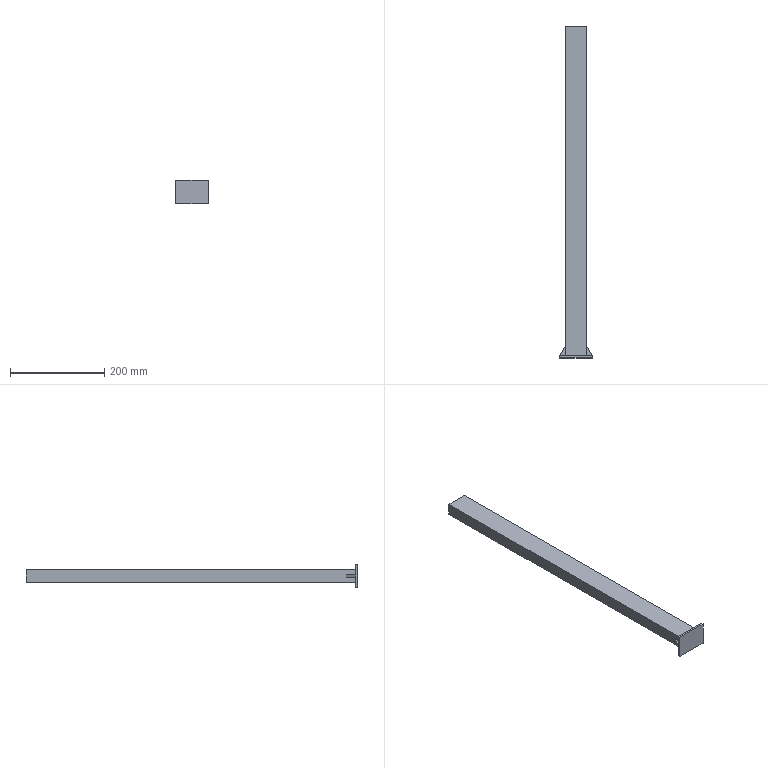Part | SolidWorks | features ICE 3, Extrusion 1 | 1 solid | 23 faces | box 70 x 705 x 50 mm | volume 217416 mm3 | plane 23
STEP:
#1=CARTESIAN_POINT('',(-415.,5.,25.));
#2=VERTEX_POINT('',#1);
#3=CARTESIAN_POINT('',(-415.,5.,2.5));
#4=VERTEX_POINT('',#3);
#5=CARTESIAN_POINT('',(-415.,5.,-25.));
#6=DIRECTION('',(0.,0.,-1.));
#7=VECTOR('',#6,1000.);
#8=LINE('',#5,#7);
#9=EDGE_CURVE('',#2,#4,#8,.T.);
#10=ORIENTED_EDGE('',*,*,#9,.T.);
#11=CARTESIAN_POINT('',(-427.,5.,2.5));
#12=VERTEX_POINT('',#11);
#13=CARTESIAN_POINT('',(-427.,5.,2.5));
#14=DIRECTION('',(1.,0.,0.));
#15=VECTOR('',#14,1000.);
#16=LINE('',#13,#15);
#17=EDGE_CURVE('',#12,#4,#16,.T.);
#18=ORIENTED_EDGE('',*,*,#17,.F.);
#19=CARTESIAN_POINT('',(-427.,5.,13.));
#20=VERTEX_POINT('',#19);
#21=CARTESIAN_POINT('',(-427.,5.,13.));
#22=DIRECTION('',(0.,0.,-1.));
#23=VECTOR('',#22,1000.);
#24=LINE('',#21,#23);
#25=EDGE_CURVE('',#20,#12,#24,.T.);
#26=ORIENTED_EDGE('',*,*,#25,.F.);
#27=CARTESIAN_POINT('',(-473.,5.,13.));
#28=VERTEX_POINT('',#27);
#29=CARTESIAN_POINT('',(-473.,5.,13.));
#30=DIRECTION('',(1.,0.,0.));
#31=VECTOR('',#30,1000.);
#32=LINE('',#29,#31);
#33=EDGE_CURVE('',#28,#20,#32,.T.);
#34=ORIENTED_EDGE('',*,*,#33,.F.);
#35=CARTESIAN_POINT('',(-473.,5.,2.5));
#36=VERTEX_POINT('',#35);
#37=CARTESIAN_POINT('',(-473.,5.,-13.));
#38=DIRECTION('',(0.,0.,1.));
#39=VECTOR('',#38,1000.);
#40=LINE('',#37,#39);
#41=EDGE_CURVE('',#36,#28,#40,.T.);
#42=ORIENTED_EDGE('',*,*,#41,.F.);
#43=CARTESIAN_POINT('',(-485.,5.,2.5));
#44=VERTEX_POINT('',#43);
#45=CARTESIAN_POINT('',(-473.,5.,2.5));
#46=DIRECTION('',(1.,0.,0.));
#47=VECTOR('',#46,1000.);
#48=LINE('',#45,#47);
#49=EDGE_CURVE('',#44,#36,#48,.T.);
#50=ORIENTED_EDGE('',*,*,#49,.F.);
#51=CARTESIAN_POINT('',(-485.,5.,25.));
#52=VERTEX_POINT('',#51);
#53=CARTESIAN_POINT('',(-485.,5.,-25.));
#54=DIRECTION('',(0.,0.,1.));
#55=VECTOR('',#54,1000.);
#56=LINE('',#53,#55);
#57=EDGE_CURVE('',#44,#52,#56,.T.);
#58=ORIENTED_EDGE('',*,*,#57,.T.);
#59=CARTESIAN_POINT('',(-485.,5.,25.));
#60=DIRECTION('',(1.,0.,0.));
#61=VECTOR('',#60,1000.);
#62=LINE('',#59,#61);
#63=EDGE_CURVE('',#52,#2,#62,.T.);
#64=ORIENTED_EDGE('',*,*,#63,.T.);
#65=EDGE_LOOP('',(#10,#18,#26,#34,#42,#50,#58,#64));
#66=FACE_OUTER_BOUND('',#65,.T.);
#67=CARTESIAN_POINT('',(0.,5.,0.));
#68=DIRECTION('',(0.,1.,0.));
#69=DIRECTION('',(0.,0.,1.));
#70=AXIS2_PLACEMENT_3D('',#67,#68,#69);
#71=PLANE('',#70);
#72=ADVANCED_FACE('',(#66),#71,.T.);
#73=CARTESIAN_POINT('',(-427.,25.,2.5));
#74=VERTEX_POINT('',#73);
#75=CARTESIAN_POINT('',(-427.,25.,2.5));
#76=DIRECTION('',(0.,-1.,0.));
#77=VECTOR('',#76,1000.);
#78=LINE('',#75,#77);
#79=EDGE_CURVE('',#74,#12,#78,.T.);
#80=ORIENTED_EDGE('',*,*,#79,.F.);
#81=CARTESIAN_POINT('',(-427.,25.,-2.5));
#82=VERTEX_POINT('',#81);
#83=CARTESIAN_POINT('',(-427.,25.,2.5));
#84=DIRECTION('',(0.,0.,-1.));
#85=VECTOR('',#84,1000.);
#86=LINE('',#83,#85);
#87=EDGE_CURVE('',#74,#82,#86,.T.);
#88=ORIENTED_EDGE('',*,*,#87,.T.);
#89=CARTESIAN_POINT('',(-427.,5.,-2.5));
#90=VERTEX_POINT('',#89);
#91=CARTESIAN_POINT('',(-427.,25.,-2.5));
#92=DIRECTION('',(0.,-1.,0.));
#93=VECTOR('',#92,1000.);
#94=LINE('',#91,#93);
#95=EDGE_CURVE('',#82,#90,#94,.T.);
#96=ORIENTED_EDGE('',*,*,#95,.T.);
#97=CARTESIAN_POINT('',(-427.,5.,-13.));
#98=VERTEX_POINT('',#97);
#99=CARTESIAN_POINT('',(-427.,5.,13.));
#100=DIRECTION('',(0.,0.,-1.));
#101=VECTOR('',#100,1000.);
#102=LINE('',#99,#101);
#103=EDGE_CURVE('',#90,#98,#102,.T.);
#104=ORIENTED_EDGE('',*,*,#103,.T.);
#105=CARTESIAN_POINT('',(-427.,705.,-13.));
#106=VERTEX_POINT('',#105);
#107=CARTESIAN_POINT('',(-427.,705.,-13.));
#108=DIRECTION('',(0.,-1.,0.));
#109=VECTOR('',#108,1000.);
#110=LINE('',#107,#109);
#111=EDGE_CURVE('',#106,#98,#110,.T.);
#112=ORIENTED_EDGE('',*,*,#111,.F.);
#113=CARTESIAN_POINT('',(-427.,705.,13.));
#114=VERTEX_POINT('',#113);
#115=CARTESIAN_POINT('',(-427.,705.,13.));
#116=DIRECTION('',(0.,0.,-1.));
#117=VECTOR('',#116,1000.);
#118=LINE('',#115,#117);
#119=EDGE_CURVE('',#114,#106,#118,.T.);
#120=ORIENTED_EDGE('',*,*,#119,.F.);
#121=CARTESIAN_POINT('',(-427.,705.,13.));
#122=DIRECTION('',(0.,-1.,0.));
#123=VECTOR('',#122,1000.);
#124=LINE('',#121,#123);
#125=EDGE_CURVE('',#114,#20,#124,.T.);
#126=ORIENTED_EDGE('',*,*,#125,.T.);
#127=ORIENTED_EDGE('',*,*,#25,.T.);
#128=EDGE_LOOP('',(#80,#88,#96,#104,#112,#120,#126,#127));
#129=FACE_OUTER_BOUND('',#128,.T.);
#130=CARTESIAN_POINT('',(-427.,705.,13.));
#131=DIRECTION('',(-1.,0.,0.));
#132=DIRECTION('',(0.,0.,1.));
#133=AXIS2_PLACEMENT_3D('',#130,#131,#132);
#134=PLANE('',#133);
#135=ADVANCED_FACE('',(#129),#134,.F.);
#136=CARTESIAN_POINT('',(-415.,5.,-2.5));
#137=VERTEX_POINT('',#136);
#138=CARTESIAN_POINT('',(-427.,5.,-2.5));
#139=DIRECTION('',(1.,0.,0.));
#140=VECTOR('',#139,1000.);
#141=LINE('',#138,#140);
#142=EDGE_CURVE('',#90,#137,#141,.T.);
#143=ORIENTED_EDGE('',*,*,#142,.T.);
#144=CARTESIAN_POINT('',(-415.,5.,-25.));
#145=VERTEX_POINT('',#144);
#146=CARTESIAN_POINT('',(-415.,5.,-25.));
#147=DIRECTION('',(0.,0.,-1.));
#148=VECTOR('',#147,1000.);
#149=LINE('',#146,#148);
#150=EDGE_CURVE('',#137,#145,#149,.T.);
#151=ORIENTED_EDGE('',*,*,#150,.T.);
#152=CARTESIAN_POINT('',(-485.,5.,-25.));
#153=VERTEX_POINT('',#152);
#154=CARTESIAN_POINT('',(-485.,5.,-25.));
#155=DIRECTION('',(-1.,0.,0.));
#156=VECTOR('',#155,1000.);
#157=LINE('',#154,#156);
#158=EDGE_CURVE('',#145,#153,#157,.T.);
#159=ORIENTED_EDGE('',*,*,#158,.T.);
#160=CARTESIAN_POINT('',(-485.,5.,-2.5));
#161=VERTEX_POINT('',#160);
#162=CARTESIAN_POINT('',(-485.,5.,-25.));
#163=DIRECTION('',(0.,0.,1.));
#164=VECTOR('',#163,1000.);
#165=LINE('',#162,#164);
#166=EDGE_CURVE('',#153,#161,#165,.T.);
#167=ORIENTED_EDGE('',*,*,#166,.T.);
#168=CARTESIAN_POINT('',(-473.,5.,-2.5));
#169=VERTEX_POINT('',#168);
#170=CARTESIAN_POINT('',(-473.,5.,-2.5));
#171=DIRECTION('',(1.,0.,0.));
#172=VECTOR('',#171,1000.);
#173=LINE('',#170,#172);
#174=EDGE_CURVE('',#161,#169,#173,.T.);
#175=ORIENTED_EDGE('',*,*,#174,.T.);
#176=CARTESIAN_POINT('',(-473.,5.,-13.));
#177=VERTEX_POINT('',#176);
#178=CARTESIAN_POINT('',(-473.,5.,-13.));
#179=DIRECTION('',(0.,0.,1.));
#180=VECTOR('',#179,1000.);
#181=LINE('',#178,#180);
#182=EDGE_CURVE('',#177,#169,#181,.T.);
#183=ORIENTED_EDGE('',*,*,#182,.F.);
#184=CARTESIAN_POINT('',(-427.,5.,-13.));
#185=DIRECTION('',(-1.,0.,0.));
#186=VECTOR('',#185,1000.);
#187=LINE('',#184,#186);
#188=EDGE_CURVE('',#98,#177,#187,.T.);
#189=ORIENTED_EDGE('',*,*,#188,.F.);
#190=ORIENTED_EDGE('',*,*,#103,.F.);
#191=EDGE_LOOP('',(#143,#151,#159,#167,#175,#183,#189,#190));
#192=FACE_OUTER_BOUND('',#191,.T.);
#193=CARTESIAN_POINT('',(0.,5.,0.));
#194=DIRECTION('',(0.,1.,0.));
#195=DIRECTION('',(0.,0.,1.));
#196=AXIS2_PLACEMENT_3D('',#193,#194,#195);
#197=PLANE('',#196);
#198=ADVANCED_FACE('',(#192),#197,.T.);
#199=CARTESIAN_POINT('',(-473.,25.,2.5));
#200=VERTEX_POINT('',#199);
#201=CARTESIAN_POINT('',(-473.,25.,2.5));
#202=DIRECTION('',(0.,1.,0.));
#203=VECTOR('',#202,1000.);
#204=LINE('',#201,#203);
#205=EDGE_CURVE('',#36,#200,#204,.T.);
#206=ORIENTED_EDGE('',*,*,#205,.F.);
#207=ORIENTED_EDGE('',*,*,#41,.T.);
#208=CARTESIAN_POINT('',(-473.,705.,13.));
#209=VERTEX_POINT('',#208);
#210=CARTESIAN_POINT('',(-473.,705.,13.));
#211=DIRECTION('',(0.,-1.,0.));
#212=VECTOR('',#211,1000.);
#213=LINE('',#210,#212);
#214=EDGE_CURVE('',#209,#28,#213,.T.);
#215=ORIENTED_EDGE('',*,*,#214,.F.);
#216=CARTESIAN_POINT('',(-473.,705.,-13.));
#217=VERTEX_POINT('',#216);
#218=CARTESIAN_POINT('',(-473.,705.,-13.));
#219=DIRECTION('',(0.,0.,1.));
#220=VECTOR('',#219,1000.);
#221=LINE('',#218,#220);
#222=EDGE_CURVE('',#217,#209,#221,.T.);
#223=ORIENTED_EDGE('',*,*,#222,.F.);
#224=CARTESIAN_POINT('',(-473.,705.,-13.));
#225=DIRECTION('',(0.,-1.,0.));
#226=VECTOR('',#225,1000.);
#227=LINE('',#224,#226);
#228=EDGE_CURVE('',#217,#177,#227,.T.);
#229=ORIENTED_EDGE('',*,*,#228,.T.);
#230=ORIENTED_EDGE('',*,*,#182,.T.);
#231=CARTESIAN_POINT('',(-473.,25.,-2.5));
#232=VERTEX_POINT('',#231);
#233=CARTESIAN_POINT('',(-473.,25.,-2.5));
#234=DIRECTION('',(0.,1.,0.));
#235=VECTOR('',#234,1000.);
#236=LINE('',#233,#235);
#237=EDGE_CURVE('',#169,#232,#236,.T.);
#238=ORIENTED_EDGE('',*,*,#237,.T.);
#239=CARTESIAN_POINT('',(-473.,25.,2.5));
#240=DIRECTION('',(0.,0.,-1.));
#241=VECTOR('',#240,1000.);
#242=LINE('',#239,#241);
#243=EDGE_CURVE('',#200,#232,#242,.T.);
#244=ORIENTED_EDGE('',*,*,#243,.F.);
#245=EDGE_LOOP('',(#206,#207,#215,#223,#229,#230,#238,#244));
#246=FACE_OUTER_BOUND('',#245,.T.);
#247=CARTESIAN_POINT('',(-473.,705.,-13.));
#248=DIRECTION('',(1.,0.,0.));
#249=DIRECTION('',(0.,0.,-1.));
#250=AXIS2_PLACEMENT_3D('',#247,#248,#249);
#251=PLANE('',#250);
#252=ADVANCED_FACE('',(#246),#251,.F.);
#253=CARTESIAN_POINT('',(-415.,0.,25.));
#254=VERTEX_POINT('',#253);
#255=CARTESIAN_POINT('',(-415.,0.,-25.));
#256=VERTEX_POINT('',#255);
#257=CARTESIAN_POINT('',(-415.,0.,-25.));
#258=DIRECTION('',(0.,0.,-1.));
#259=VECTOR('',#258,1000.);
#260=LINE('',#257,#259);
#261=EDGE_CURVE('',#254,#256,#260,.T.);
#262=ORIENTED_EDGE('',*,*,#261,.T.);
#263=CARTESIAN_POINT('',(-415.,5.,-25.));
#264=DIRECTION('',(0.,-1.,0.));
#265=VECTOR('',#264,1000.);
#266=LINE('',#263,#265);
#267=EDGE_CURVE('',#145,#256,#266,.T.);
#268=ORIENTED_EDGE('',*,*,#267,.F.);
#269=ORIENTED_EDGE('',*,*,#150,.F.);
#270=CARTESIAN_POINT('',(-415.,5.,2.5));
#271=DIRECTION('',(0.,0.,-1.));
#272=VECTOR('',#271,1000.);
#273=LINE('',#270,#272);
#274=EDGE_CURVE('',#4,#137,#273,.T.);
#275=ORIENTED_EDGE('',*,*,#274,.F.);
#276=ORIENTED_EDGE('',*,*,#9,.F.);
#277=CARTESIAN_POINT('',(-415.,5.,25.));
#278=DIRECTION('',(0.,-1.,0.));
#279=VECTOR('',#278,1000.);
#280=LINE('',#277,#279);
#281=EDGE_CURVE('',#2,#254,#280,.T.);
#282=ORIENTED_EDGE('',*,*,#281,.T.);
#283=EDGE_LOOP('',(#262,#268,#269,#275,#276,#282));
#284=FACE_OUTER_BOUND('',#283,.T.);
#285=CARTESIAN_POINT('',(-415.,5.,-25.));
#286=DIRECTION('',(-1.,0.,0.));
#287=DIRECTION('',(0.,0.,1.));
#288=AXIS2_PLACEMENT_3D('',#285,#286,#287);
#289=PLANE('',#288);
#290=ADVANCED_FACE('',(#284),#289,.F.);
#291=CARTESIAN_POINT('',(-485.,0.,-25.));
#292=VERTEX_POINT('',#291);
#293=CARTESIAN_POINT('',(-485.,0.,-25.));
#294=DIRECTION('',(-1.,0.,0.));
#295=VECTOR('',#294,1000.);
#296=LINE('',#293,#295);
#297=EDGE_CURVE('',#256,#292,#296,.T.);
#298=ORIENTED_EDGE('',*,*,#297,.T.);
#299=CARTESIAN_POINT('',(-485.,5.,-25.));
#300=DIRECTION('',(0.,-1.,0.));
#301=VECTOR('',#300,1000.);
#302=LINE('',#299,#301);
#303=EDGE_CURVE('',#153,#292,#302,.T.);
#304=ORIENTED_EDGE('',*,*,#303,.F.);
#305=ORIENTED_EDGE('',*,*,#158,.F.);
#306=ORIENTED_EDGE('',*,*,#267,.T.);
#307=EDGE_LOOP('',(#298,#304,#305,#306));
#308=FACE_OUTER_BOUND('',#307,.T.);
#309=CARTESIAN_POINT('',(-485.,5.,-25.));
#310=DIRECTION('',(0.,0.,1.));
#311=DIRECTION('',(1.,0.,0.));
#312=AXIS2_PLACEMENT_3D('',#309,#310,#311);
#313=PLANE('',#312);
#314=ADVANCED_FACE('',(#308),#313,.F.);
#315=CARTESIAN_POINT('',(-485.,0.,25.));
#316=VERTEX_POINT('',#315);
#317=CARTESIAN_POINT('',(-485.,0.,-25.));
#318=DIRECTION('',(0.,0.,1.));
#319=VECTOR('',#318,1000.);
#320=LINE('',#317,#319);
#321=EDGE_CURVE('',#292,#316,#320,.T.);
#322=ORIENTED_EDGE('',*,*,#321,.T.);
#323=CARTESIAN_POINT('',(-485.,5.,25.));
#324=DIRECTION('',(0.,-1.,0.));
#325=VECTOR('',#324,1000.);
#326=LINE('',#323,#325);
#327=EDGE_CURVE('',#52,#316,#326,.T.);
#328=ORIENTED_EDGE('',*,*,#327,.F.);
#329=ORIENTED_EDGE('',*,*,#57,.F.);
#330=CARTESIAN_POINT('',(-485.,5.,2.5));
#331=DIRECTION('',(0.,0.,-1.));
#332=VECTOR('',#331,1000.);
#333=LINE('',#330,#332);
#334=EDGE_CURVE('',#44,#161,#333,.T.);
#335=ORIENTED_EDGE('',*,*,#334,.T.);
#336=ORIENTED_EDGE('',*,*,#166,.F.);
#337=ORIENTED_EDGE('',*,*,#303,.T.);
#338=EDGE_LOOP('',(#322,#328,#329,#335,#336,#337));
#339=FACE_OUTER_BOUND('',#338,.T.);
#340=CARTESIAN_POINT('',(-485.,5.,-25.));
#341=DIRECTION('',(1.,0.,0.));
#342=DIRECTION('',(0.,0.,-1.));
#343=AXIS2_PLACEMENT_3D('',#340,#341,#342);
#344=PLANE('',#343);
#345=ADVANCED_FACE('',(#339),#344,.F.);
#346=CARTESIAN_POINT('',(-485.,0.,25.));
#347=DIRECTION('',(1.,0.,0.));
#348=VECTOR('',#347,1000.);
#349=LINE('',#346,#348);
#350=EDGE_CURVE('',#316,#254,#349,.T.);
#351=ORIENTED_EDGE('',*,*,#350,.T.);
#352=ORIENTED_EDGE('',*,*,#281,.F.);
#353=ORIENTED_EDGE('',*,*,#63,.F.);
#354=ORIENTED_EDGE('',*,*,#327,.T.);
#355=EDGE_LOOP('',(#351,#352,#353,#354));
#356=FACE_OUTER_BOUND('',#355,.T.);
#357=CARTESIAN_POINT('',(-485.,5.,25.));
#358=DIRECTION('',(0.,0.,-1.));
#359=DIRECTION('',(-1.,0.,0.));
#360=AXIS2_PLACEMENT_3D('',#357,#358,#359);
#361=PLANE('',#360);
#362=ADVANCED_FACE('',(#356),#361,.F.);
#363=ORIENTED_EDGE('',*,*,#261,.F.);
#364=ORIENTED_EDGE('',*,*,#350,.F.);
#365=ORIENTED_EDGE('',*,*,#321,.F.);
#366=ORIENTED_EDGE('',*,*,#297,.F.);
#367=EDGE_LOOP('',(#363,#364,#365,#366));
#368=FACE_OUTER_BOUND('',#367,.T.);
#369=CARTESIAN_POINT('',(0.,0.,0.));
#370=DIRECTION('',(0.,1.,0.));
#371=DIRECTION('',(0.,0.,1.));
#372=AXIS2_PLACEMENT_3D('',#369,#370,#371);
#373=PLANE('',#372);
#374=ADVANCED_FACE('',(#368),#373,.F.);
#375=ORIENTED_EDGE('',*,*,#33,.T.);
#376=ORIENTED_EDGE('',*,*,#125,.F.);
#377=CARTESIAN_POINT('',(-473.,705.,13.));
#378=DIRECTION('',(1.,0.,0.));
#379=VECTOR('',#378,1000.);
#380=LINE('',#377,#379);
#381=EDGE_CURVE('',#209,#114,#380,.T.);
#382=ORIENTED_EDGE('',*,*,#381,.F.);
#383=ORIENTED_EDGE('',*,*,#214,.T.);
#384=EDGE_LOOP('',(#375,#376,#382,#383));
#385=FACE_OUTER_BOUND('',#384,.T.);
#386=CARTESIAN_POINT('',(-473.,705.,13.));
#387=DIRECTION('',(0.,0.,-1.));
#388=DIRECTION('',(-1.,0.,0.));
#389=AXIS2_PLACEMENT_3D('',#386,#387,#388);
#390=PLANE('',#389);
#391=ADVANCED_FACE('',(#385),#390,.F.);
#392=ORIENTED_EDGE('',*,*,#188,.T.);
#393=ORIENTED_EDGE('',*,*,#228,.F.);
#394=CARTESIAN_POINT('',(-427.,705.,-13.));
#395=DIRECTION('',(-1.,0.,0.));
#396=VECTOR('',#395,1000.);
#397=LINE('',#394,#396);
#398=EDGE_CURVE('',#106,#217,#397,.T.);
#399=ORIENTED_EDGE('',*,*,#398,.F.);
#400=ORIENTED_EDGE('',*,*,#111,.T.);
#401=EDGE_LOOP('',(#392,#393,#399,#400));
#402=FACE_OUTER_BOUND('',#401,.T.);
#403=CARTESIAN_POINT('',(-427.,705.,-13.));
#404=DIRECTION('',(0.,0.,1.));
#405=DIRECTION('',(1.,0.,0.));
#406=AXIS2_PLACEMENT_3D('',#403,#404,#405);
#407=PLANE('',#406);
#408=ADVANCED_FACE('',(#402),#407,.F.);
#409=CARTESIAN_POINT('',(-471.,705.,-11.));
#410=VERTEX_POINT('',#409);
#411=CARTESIAN_POINT('',(-471.,705.,11.));
#412=VERTEX_POINT('',#411);
#413=CARTESIAN_POINT('',(-471.,705.,-11.));
#414=DIRECTION('',(0.,0.,1.));
#415=VECTOR('',#414,1000.);
#416=LINE('',#413,#415);
#417=EDGE_CURVE('',#410,#412,#416,.T.);
#418=ORIENTED_EDGE('',*,*,#417,.F.);
#419=CARTESIAN_POINT('',(-429.,705.,-11.));
#420=VERTEX_POINT('',#419);
#421=CARTESIAN_POINT('',(-429.,705.,-11.));
#422=DIRECTION('',(-1.,0.,0.));
#423=VECTOR('',#422,1000.);
#424=LINE('',#421,#423);
#425=EDGE_CURVE('',#420,#410,#424,.T.);
#426=ORIENTED_EDGE('',*,*,#425,.F.);
#427=CARTESIAN_POINT('',(-429.,705.,11.));
#428=VERTEX_POINT('',#427);
#429=CARTESIAN_POINT('',(-429.,705.,11.));
#430=DIRECTION('',(0.,0.,-1.));
#431=VECTOR('',#430,1000.);
#432=LINE('',#429,#431);
#433=EDGE_CURVE('',#428,#420,#432,.T.);
#434=ORIENTED_EDGE('',*,*,#433,.F.);
#435=CARTESIAN_POINT('',(-471.,705.,11.));
#436=DIRECTION('',(1.,0.,0.));
#437=VECTOR('',#436,1000.);
#438=LINE('',#435,#437);
#439=EDGE_CURVE('',#412,#428,#438,.T.);
#440=ORIENTED_EDGE('',*,*,#439,.F.);
#441=EDGE_LOOP('',(#418,#426,#434,#440));
#442=FACE_BOUND('',#441,.T.);
#443=ORIENTED_EDGE('',*,*,#381,.T.);
#444=ORIENTED_EDGE('',*,*,#119,.T.);
#445=ORIENTED_EDGE('',*,*,#398,.T.);
#446=ORIENTED_EDGE('',*,*,#222,.T.);
#447=EDGE_LOOP('',(#443,#444,#445,#446));
#448=FACE_OUTER_BOUND('',#447,.T.);
#449=CARTESIAN_POINT('',(0.,705.,0.));
#450=DIRECTION('',(0.,1.,0.));
#451=DIRECTION('',(0.,0.,1.));
#452=AXIS2_PLACEMENT_3D('',#449,#450,#451);
#453=PLANE('',#452);
#454=ADVANCED_FACE('',(#442,#448),#453,.T.);
#455=CARTESIAN_POINT('',(-485.,5.,-2.5));
#456=DIRECTION('',(-0.5145,-0.8575,0.));
#457=VECTOR('',#456,1000.);
#458=LINE('',#455,#457);
#459=EDGE_CURVE('',#232,#161,#458,.T.);
#460=ORIENTED_EDGE('',*,*,#459,.T.);
#461=ORIENTED_EDGE('',*,*,#334,.F.);
#462=CARTESIAN_POINT('',(-485.,5.,2.5));
#463=DIRECTION('',(-0.5145,-0.8575,0.));
#464=VECTOR('',#463,1000.);
#465=LINE('',#462,#464);
#466=EDGE_CURVE('',#200,#44,#465,.T.);
#467=ORIENTED_EDGE('',*,*,#466,.F.);
#468=ORIENTED_EDGE('',*,*,#243,.T.);
#469=EDGE_LOOP('',(#460,#461,#467,#468));
#470=FACE_OUTER_BOUND('',#469,.T.);
#471=CARTESIAN_POINT('',(-485.,5.,2.5));
#472=DIRECTION('',(0.8575,-0.5145,0.));
#473=DIRECTION('',(0.5145,0.8575,0.));
#474=AXIS2_PLACEMENT_3D('',#471,#472,#473);
#475=PLANE('',#474);
#476=ADVANCED_FACE('',(#470),#475,.F.);
#477=ORIENTED_EDGE('',*,*,#205,.T.);
#478=ORIENTED_EDGE('',*,*,#466,.T.);
#479=ORIENTED_EDGE('',*,*,#49,.T.);
#480=EDGE_LOOP('',(#477,#478,#479));
#481=FACE_OUTER_BOUND('',#480,.T.);
#482=CARTESIAN_POINT('',(0.,0.,2.5));
#483=DIRECTION('',(0.,0.,-1.));
#484=DIRECTION('',(-1.,0.,0.));
#485=AXIS2_PLACEMENT_3D('',#482,#483,#484);
#486=PLANE('',#485);
#487=ADVANCED_FACE('',(#481),#486,.F.);
#488=ORIENTED_EDGE('',*,*,#237,.F.);
#489=ORIENTED_EDGE('',*,*,#174,.F.);
#490=ORIENTED_EDGE('',*,*,#459,.F.);
#491=EDGE_LOOP('',(#488,#489,#490));
#492=FACE_OUTER_BOUND('',#491,.T.);
#493=CARTESIAN_POINT('',(0.,0.,-2.5));
#494=DIRECTION('',(0.,0.,-1.));
#495=DIRECTION('',(-1.,0.,0.));
#496=AXIS2_PLACEMENT_3D('',#493,#494,#495);
#497=PLANE('',#496);
#498=ADVANCED_FACE('',(#492),#497,.T.);
#499=CARTESIAN_POINT('',(-415.,5.,-2.5));
#500=DIRECTION('',(-0.5145,0.8575,0.));
#501=VECTOR('',#500,1000.);
#502=LINE('',#499,#501);
#503=EDGE_CURVE('',#137,#82,#502,.T.);
#504=ORIENTED_EDGE('',*,*,#503,.T.);
#505=ORIENTED_EDGE('',*,*,#87,.F.);
#506=CARTESIAN_POINT('',(-415.,5.,2.5));
#507=DIRECTION('',(-0.5145,0.8575,0.));
#508=VECTOR('',#507,1000.);
#509=LINE('',#506,#508);
#510=EDGE_CURVE('',#4,#74,#509,.T.);
#511=ORIENTED_EDGE('',*,*,#510,.F.);
#512=ORIENTED_EDGE('',*,*,#274,.T.);
#513=EDGE_LOOP('',(#504,#505,#511,#512));
#514=FACE_OUTER_BOUND('',#513,.T.);
#515=CARTESIAN_POINT('',(-415.,5.,2.5));
#516=DIRECTION('',(-0.8575,-0.5145,0.));
#517=DIRECTION('',(0.5145,-0.8575,0.));
#518=AXIS2_PLACEMENT_3D('',#515,#516,#517);
#519=PLANE('',#518);
#520=ADVANCED_FACE('',(#514),#519,.F.);
#521=ORIENTED_EDGE('',*,*,#510,.T.);
#522=ORIENTED_EDGE('',*,*,#79,.T.);
#523=ORIENTED_EDGE('',*,*,#17,.T.);
#524=EDGE_LOOP('',(#521,#522,#523));
#525=FACE_OUTER_BOUND('',#524,.T.);
#526=CARTESIAN_POINT('',(0.,0.,2.5));
#527=DIRECTION('',(0.,0.,-1.));
#528=DIRECTION('',(-1.,0.,0.));
#529=AXIS2_PLACEMENT_3D('',#526,#527,#528);
#530=PLANE('',#529);
#531=ADVANCED_FACE('',(#525),#530,.F.);
#532=ORIENTED_EDGE('',*,*,#503,.F.);
#533=ORIENTED_EDGE('',*,*,#142,.F.);
#534=ORIENTED_EDGE('',*,*,#95,.F.);
#535=EDGE_LOOP('',(#532,#533,#534));
#536=FACE_OUTER_BOUND('',#535,.T.);
#537=CARTESIAN_POINT('',(0.,0.,-2.5));
#538=DIRECTION('',(0.,0.,-1.));
#539=DIRECTION('',(-1.,0.,0.));
#540=AXIS2_PLACEMENT_3D('',#537,#538,#539);
#541=PLANE('',#540);
#542=ADVANCED_FACE('',(#536),#541,.T.);
#543=ORIENTED_EDGE('',*,*,#417,.T.);
#544=CARTESIAN_POINT('',(-471.,14.,11.));
#545=VERTEX_POINT('',#544);
#546=CARTESIAN_POINT('',(-471.,14.,11.));
#547=DIRECTION('',(0.,1.,0.));
#548=VECTOR('',#547,1000.);
#549=LINE('',#546,#548);
#550=EDGE_CURVE('',#545,#412,#549,.T.);
#551=ORIENTED_EDGE('',*,*,#550,.F.);
#552=CARTESIAN_POINT('',(-471.,14.,-11.));
#553=VERTEX_POINT('',#552);
#554=CARTESIAN_POINT('',(-471.,14.,-11.));
#555=DIRECTION('',(0.,0.,1.));
#556=VECTOR('',#555,1000.);
#557=LINE('',#554,#556);
#558=EDGE_CURVE('',#553,#545,#557,.T.);
#559=ORIENTED_EDGE('',*,*,#558,.F.);
#560=CARTESIAN_POINT('',(-471.,14.,-11.));
#561=DIRECTION('',(0.,1.,0.));
#562=VECTOR('',#561,1000.);
#563=LINE('',#560,#562);
#564=EDGE_CURVE('',#553,#410,#563,.T.);
#565=ORIENTED_EDGE('',*,*,#564,.T.);
#566=EDGE_LOOP('',(#543,#551,#559,#565));
#567=FACE_OUTER_BOUND('',#566,.T.);
#568=CARTESIAN_POINT('',(-471.,14.,-11.));
#569=DIRECTION('',(-1.,0.,0.));
#570=DIRECTION('',(0.,0.,1.));
#571=AXIS2_PLACEMENT_3D('',#568,#569,#570);
#572=PLANE('',#571);
#573=ADVANCED_FACE('',(#567),#572,.F.);
#574=ORIENTED_EDGE('',*,*,#425,.T.);
#575=ORIENTED_EDGE('',*,*,#564,.F.);
#576=CARTESIAN_POINT('',(-429.,14.,-11.));
#577=VERTEX_POINT('',#576);
#578=CARTESIAN_POINT('',(-429.,14.,-11.));
#579=DIRECTION('',(-1.,0.,0.));
#580=VECTOR('',#579,1000.);
#581=LINE('',#578,#580);
#582=EDGE_CURVE('',#577,#553,#581,.T.);
#583=ORIENTED_EDGE('',*,*,#582,.F.);
#584=CARTESIAN_POINT('',(-429.,14.,-11.));
#585=DIRECTION('',(0.,1.,0.));
#586=VECTOR('',#585,1000.);
#587=LINE('',#584,#586);
#588=EDGE_CURVE('',#577,#420,#587,.T.);
#589=ORIENTED_EDGE('',*,*,#588,.T.);
#590=EDGE_LOOP('',(#574,#575,#583,#589));
#591=FACE_OUTER_BOUND('',#590,.T.);
#592=CARTESIAN_POINT('',(-429.,14.,-11.));
#593=DIRECTION('',(0.,0.,-1.));
#594=DIRECTION('',(-1.,0.,0.));
#595=AXIS2_PLACEMENT_3D('',#592,#593,#594);
#596=PLANE('',#595);
#597=ADVANCED_FACE('',(#591),#596,.F.);
#598=ORIENTED_EDGE('',*,*,#433,.T.);
#599=ORIENTED_EDGE('',*,*,#588,.F.);
#600=CARTESIAN_POINT('',(-429.,14.,11.));
#601=VERTEX_POINT('',#600);
#602=CARTESIAN_POINT('',(-429.,14.,11.));
#603=DIRECTION('',(0.,0.,-1.));
#604=VECTOR('',#603,1000.);
#605=LINE('',#602,#604);
#606=EDGE_CURVE('',#601,#577,#605,.T.);
#607=ORIENTED_EDGE('',*,*,#606,.F.);
#608=CARTESIAN_POINT('',(-429.,14.,11.));
#609=DIRECTION('',(0.,1.,0.));
#610=VECTOR('',#609,1000.);
#611=LINE('',#608,#610);
#612=EDGE_CURVE('',#601,#428,#611,.T.);
#613=ORIENTED_EDGE('',*,*,#612,.T.);
#614=EDGE_LOOP('',(#598,#599,#607,#613));
#615=FACE_OUTER_BOUND('',#614,.T.);
#616=CARTESIAN_POINT('',(-429.,14.,11.));
#617=DIRECTION('',(1.,0.,0.));
#618=DIRECTION('',(0.,0.,-1.));
#619=AXIS2_PLACEMENT_3D('',#616,#617,#618);
#620=PLANE('',#619);
#621=ADVANCED_FACE('',(#615),#620,.F.);
#622=ORIENTED_EDGE('',*,*,#439,.T.);
#623=ORIENTED_EDGE('',*,*,#612,.F.);
#624=CARTESIAN_POINT('',(-471.,14.,11.));
#625=DIRECTION('',(1.,0.,0.));
#626=VECTOR('',#625,1000.);
#627=LINE('',#624,#626);
#628=EDGE_CURVE('',#545,#601,#627,.T.);
#629=ORIENTED_EDGE('',*,*,#628,.F.);
#630=ORIENTED_EDGE('',*,*,#550,.T.);
#631=EDGE_LOOP('',(#622,#623,#629,#630));
#632=FACE_OUTER_BOUND('',#631,.T.);
#633=CARTESIAN_POINT('',(-471.,14.,11.));
#634=DIRECTION('',(0.,0.,1.));
#635=DIRECTION('',(1.,0.,0.));
#636=AXIS2_PLACEMENT_3D('',#633,#634,#635);
#637=PLANE('',#636);
#638=ADVANCED_FACE('',(#632),#637,.F.);
#639=ORIENTED_EDGE('',*,*,#558,.T.);
#640=ORIENTED_EDGE('',*,*,#628,.T.);
#641=ORIENTED_EDGE('',*,*,#606,.T.);
#642=ORIENTED_EDGE('',*,*,#582,.T.);
#643=EDGE_LOOP('',(#639,#640,#641,#642));
#644=FACE_OUTER_BOUND('',#643,.T.);
#645=CARTESIAN_POINT('',(0.,14.,0.));
#646=DIRECTION('',(0.,1.,0.));
#647=DIRECTION('',(0.,0.,1.));
#648=AXIS2_PLACEMENT_3D('',#645,#646,#647);
#649=PLANE('',#648);
#650=ADVANCED_FACE('',(#644),#649,.T.);
#651=CLOSED_SHELL('',(#72,#135,#198,#252,#290,#314,#345,#362,#374,#391,#408,#454,#476,#487,#498,#520,#531,#542,#573,#597,#621,#638,#650));
#652=MANIFOLD_SOLID_BREP('',#651);
#653=CARTESIAN_POINT('',(0.,0.,0.));
#654=DIRECTION('',(0.,0.,1.));
#655=DIRECTION('',(1.,0.,0.));
#656=AXIS2_PLACEMENT_3D('',#653,#654,#655);
#657=(LENGTH_UNIT()NAMED_UNIT(*)SI_UNIT(.MILLI.,.METRE.));
#658=UNCERTAINTY_MEASURE_WITH_UNIT(LENGTH_MEASURE(0.00001),#657,'','');
#659=(NAMED_UNIT(*)PLANE_ANGLE_UNIT()SI_UNIT($,.RADIAN.));
#660=(NAMED_UNIT(*)SI_UNIT($,.STERADIAN.)SOLID_ANGLE_UNIT());
#661=(GEOMETRIC_REPRESENTATION_CONTEXT(3)GLOBAL_UNCERTAINTY_ASSIGNED_CONTEXT((#658))GLOBAL_UNIT_ASSIGNED_CONTEXT((#657,#659,#660))REPRESENTATION_CONTEXT('',''));
#662=ADVANCED_BREP_SHAPE_REPRESENTATION('',(#652,#656),#661);